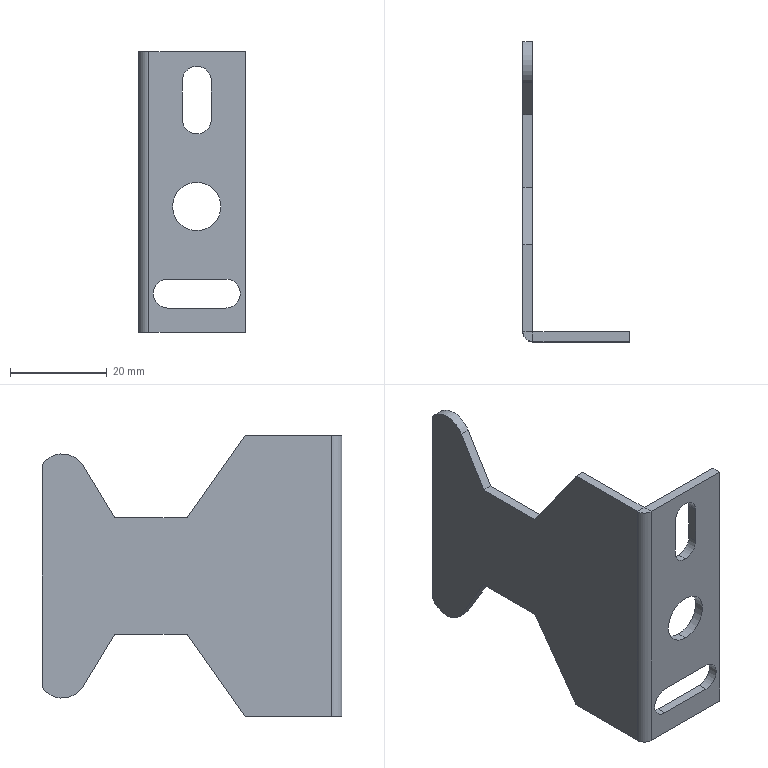Part | STEP file | Photoelectric bracket 2 | 1 solid | 33 faces | box 22 x 62 x 58 mm | volume 7067 mm3 | plane 22 | cylinder 11 | commonest cylinder face diameters 6 x5 10 x4 0.2 x1 4.2 x1